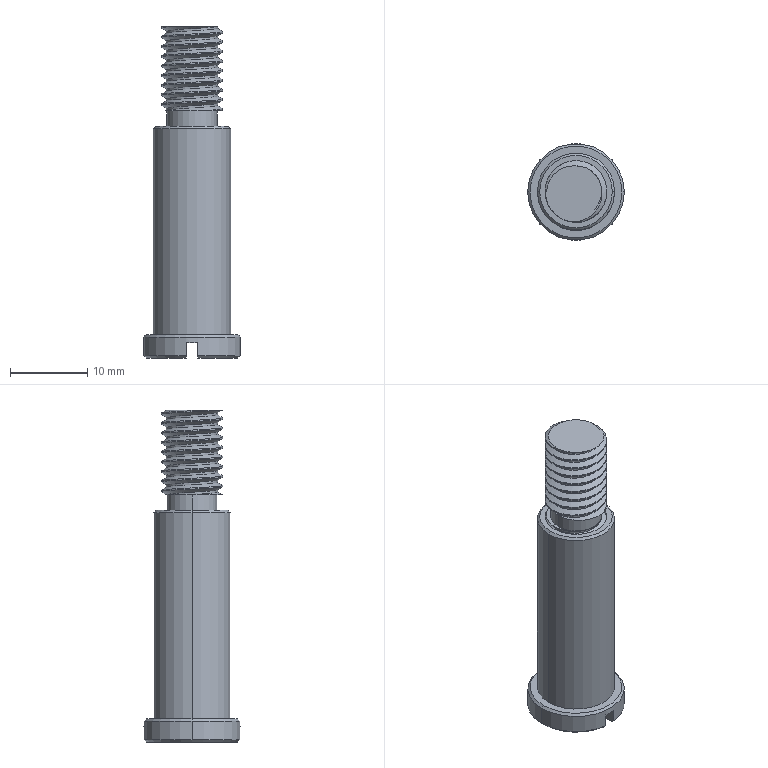Part | SolidWorks | features BaseBody 1 | 1 solid | 50 faces | box 12.5 x 12.5 x 43 mm | volume 2962 mm3 | cylinder 25 | plane 11 | cone 7 | spline 7 | commonest cylinder face diameters 8 x19 6.5 x2 10 x2 12.5 x2